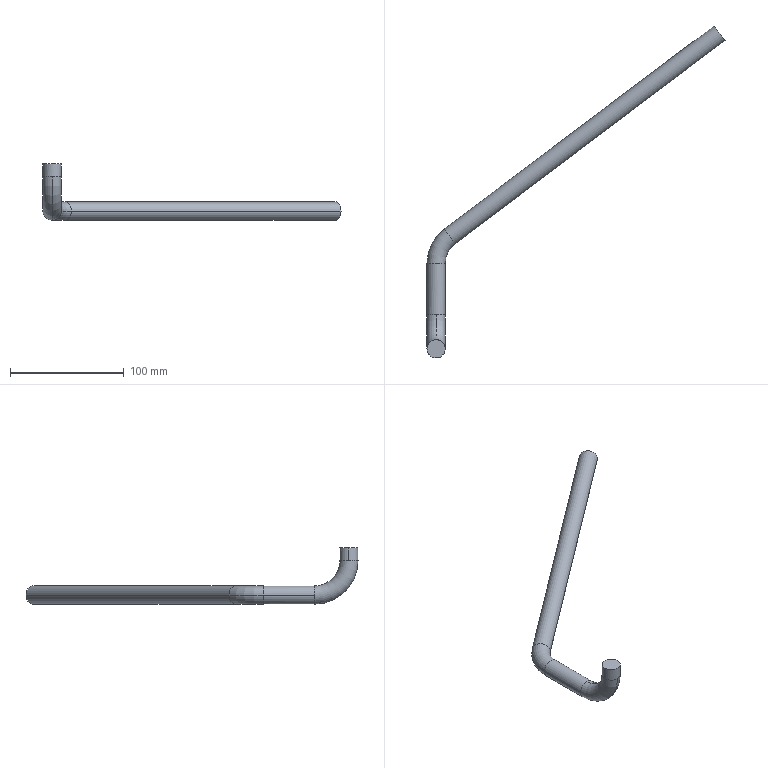Part | STEP file | copper tube 37 | 1 solid | 12 faces | box 261.823 x 291.69 x 49.416 mm | volume 86044 mm3 | cylinder 6 | torus 4 | plane 2 | commonest cylinder face diameters 16 x6
STEP:
#1=CARTESIAN_POINT('',(0.,0.,0.));
#2=DIRECTION('',(0.,0.,1.));
#3=DIRECTION('',(1.,0.,0.));
#4=AXIS2_PLACEMENT_3D('',#1,#2,#3);
#5=CARTESIAN_POINT('',(0.,-8.,-61.416));
#6=VERTEX_POINT('',#5);
#7=CARTESIAN_POINT('',(8.,0.,-61.416));
#8=VERTEX_POINT('',#7);
#9=CARTESIAN_POINT('',(0.,0.,-61.416));
#10=DIRECTION('',(0.,0.,1.));
#11=DIRECTION('',(1.,0.,0.));
#12=AXIS2_PLACEMENT_3D('',#9,#10,#11);
#13=CIRCLE('',#12,8.);
#14=CARTESIAN_POINT('',(0.,30.,-61.416));
#15=DIRECTION('',(1.,0.,0.));
#16=DIRECTION('',(0.,1.,0.));
#17=AXIS2_PLACEMENT_3D('',#14,#15,#16);
#18=TOROIDAL_SURFACE('',#17,30.,8.);
#19=CARTESIAN_POINT('',(3.142,-4.712));
#20=DIRECTION('',(0.,1.));
#21=VECTOR('',#20,1.);
#22=LINE('',#19,#21);
#23=(GEOMETRIC_REPRESENTATION_CONTEXT(2)PARAMETRIC_REPRESENTATION_CONTEXT()REPRESENTATION_CONTEXT('',''));
#24=DEFINITIONAL_REPRESENTATION('',(#22),#23);
#25=PCURVE('',#18,#24);
#26=CARTESIAN_POINT('',(0.,0.,-61.416));
#27=DIRECTION('',(0.,0.,1.));
#28=DIRECTION('',(1.,0.,0.));
#29=AXIS2_PLACEMENT_3D('',#26,#27,#28);
#30=CYLINDRICAL_SURFACE('',#29,8.);
#31=CARTESIAN_POINT('',(0.,0.));
#32=DIRECTION('',(1.,0.));
#33=VECTOR('',#32,1.);
#34=LINE('',#31,#33);
#35=(GEOMETRIC_REPRESENTATION_CONTEXT(2)PARAMETRIC_REPRESENTATION_CONTEXT()REPRESENTATION_CONTEXT('',''));
#36=DEFINITIONAL_REPRESENTATION('',(#34),#35);
#37=PCURVE('',#30,#36);
#38=SURFACE_CURVE('',#13,(#25,#37),.PCURVE_S1.);
#39=EDGE_CURVE('',#6,#8,#38,.T.);
#40=ORIENTED_EDGE('',*,*,#39,.F.);
#41=CARTESIAN_POINT('',(0.,30.,-99.416));
#42=VERTEX_POINT('',#41);
#43=CARTESIAN_POINT('',(0.,30.,-61.416));
#44=DIRECTION('',(1.,0.,0.));
#45=DIRECTION('',(0.,1.,0.));
#46=AXIS2_PLACEMENT_3D('',#43,#44,#45);
#47=CIRCLE('',#46,38.);
#48=CARTESIAN_POINT('',(0.,0.));
#49=DIRECTION('',(1.,0.));
#50=VECTOR('',#49,1.);
#51=LINE('',#48,#50);
#52=(GEOMETRIC_REPRESENTATION_CONTEXT(2)PARAMETRIC_REPRESENTATION_CONTEXT()REPRESENTATION_CONTEXT('',''));
#53=DEFINITIONAL_REPRESENTATION('',(#51),#52);
#54=PCURVE('',#18,#53);
#55=CARTESIAN_POINT('',(0.,30.,-61.416));
#56=DIRECTION('',(1.,0.,0.));
#57=DIRECTION('',(0.,1.,0.));
#58=AXIS2_PLACEMENT_3D('',#55,#56,#57);
#59=TOROIDAL_SURFACE('',#58,30.,8.);
#60=CARTESIAN_POINT('',(0.,6.283));
#61=DIRECTION('',(1.,0.));
#62=VECTOR('',#61,1.);
#63=LINE('',#60,#62);
#64=(GEOMETRIC_REPRESENTATION_CONTEXT(2)PARAMETRIC_REPRESENTATION_CONTEXT()REPRESENTATION_CONTEXT('',''));
#65=DEFINITIONAL_REPRESENTATION('',(#63),#64);
#66=PCURVE('',#59,#65);
#67=SURFACE_CURVE('',#47,(#54,#66),.PCURVE_S1.);
#68=EDGE_CURVE('',#6,#42,#67,.T.);
#69=ORIENTED_EDGE('',*,*,#68,.T.);
#70=CARTESIAN_POINT('',(8.,30.,-91.416));
#71=VERTEX_POINT('',#70);
#72=CARTESIAN_POINT('',(0.,30.,-91.416));
#73=DIRECTION('',(0.,-1.,0.));
#74=DIRECTION('',(1.,0.,0.));
#75=AXIS2_PLACEMENT_3D('',#72,#73,#74);
#76=CIRCLE('',#75,8.);
#77=CARTESIAN_POINT('',(4.712,-4.712));
#78=DIRECTION('',(0.,1.));
#79=VECTOR('',#78,1.);
#80=LINE('',#77,#79);
#81=(GEOMETRIC_REPRESENTATION_CONTEXT(2)PARAMETRIC_REPRESENTATION_CONTEXT()REPRESENTATION_CONTEXT('',''));
#82=DEFINITIONAL_REPRESENTATION('',(#80),#81);
#83=PCURVE('',#18,#82);
#84=CARTESIAN_POINT('',(0.,30.,-91.416));
#85=DIRECTION('',(0.,1.,0.));
#86=DIRECTION('',(-1.,0.,0.));
#87=AXIS2_PLACEMENT_3D('',#84,#85,#86);
#88=CYLINDRICAL_SURFACE('',#87,8.);
#89=CARTESIAN_POINT('',(9.425,0.));
#90=DIRECTION('',(-1.,0.));
#91=VECTOR('',#90,1.);
#92=LINE('',#89,#91);
#93=(GEOMETRIC_REPRESENTATION_CONTEXT(2)PARAMETRIC_REPRESENTATION_CONTEXT()REPRESENTATION_CONTEXT('',''));
#94=DEFINITIONAL_REPRESENTATION('',(#92),#93);
#95=PCURVE('',#88,#94);
#96=SURFACE_CURVE('',#76,(#83,#95),.PCURVE_S1.);
#97=EDGE_CURVE('',#42,#71,#96,.T.);
#98=ORIENTED_EDGE('',*,*,#97,.T.);
#99=CARTESIAN_POINT('',(0.,30.,-83.416));
#100=VERTEX_POINT('',#99);
#101=CARTESIAN_POINT('',(0.,30.,-91.416));
#102=DIRECTION('',(0.,-1.,0.));
#103=DIRECTION('',(1.,0.,0.));
#104=AXIS2_PLACEMENT_3D('',#101,#102,#103);
#105=CIRCLE('',#104,8.);
#106=CARTESIAN_POINT('',(4.712,1.571));
#107=DIRECTION('',(0.,1.));
#108=VECTOR('',#107,1.);
#109=LINE('',#106,#108);
#110=(GEOMETRIC_REPRESENTATION_CONTEXT(2)PARAMETRIC_REPRESENTATION_CONTEXT()REPRESENTATION_CONTEXT('',''));
#111=DEFINITIONAL_REPRESENTATION('',(#109),#110);
#112=PCURVE('',#18,#111);
#113=CARTESIAN_POINT('',(0.,30.,-91.416));
#114=DIRECTION('',(0.,1.,0.));
#115=DIRECTION('',(-1.,0.,0.));
#116=AXIS2_PLACEMENT_3D('',#113,#114,#115);
#117=CYLINDRICAL_SURFACE('',#116,8.);
#118=CARTESIAN_POINT('',(3.142,0.));
#119=DIRECTION('',(-1.,0.));
#120=VECTOR('',#119,1.);
#121=LINE('',#118,#120);
#122=(GEOMETRIC_REPRESENTATION_CONTEXT(2)PARAMETRIC_REPRESENTATION_CONTEXT()REPRESENTATION_CONTEXT('',''));
#123=DEFINITIONAL_REPRESENTATION('',(#121),#122);
#124=PCURVE('',#117,#123);
#125=SURFACE_CURVE('',#105,(#112,#124),.PCURVE_S1.);
#126=EDGE_CURVE('',#71,#100,#125,.T.);
#127=ORIENTED_EDGE('',*,*,#126,.T.);
#128=CARTESIAN_POINT('',(0.,8.,-61.416));
#129=VERTEX_POINT('',#128);
#130=CARTESIAN_POINT('',(0.,30.,-61.416));
#131=DIRECTION('',(1.,0.,0.));
#132=DIRECTION('',(0.,1.,0.));
#133=AXIS2_PLACEMENT_3D('',#130,#131,#132);
#134=CIRCLE('',#133,22.);
#135=CARTESIAN_POINT('',(0.,3.142));
#136=DIRECTION('',(1.,0.));
#137=VECTOR('',#136,1.);
#138=LINE('',#135,#137);
#139=(GEOMETRIC_REPRESENTATION_CONTEXT(2)PARAMETRIC_REPRESENTATION_CONTEXT()REPRESENTATION_CONTEXT('',''));
#140=DEFINITIONAL_REPRESENTATION('',(#138),#139);
#141=PCURVE('',#18,#140);
#142=CARTESIAN_POINT('',(0.,3.142));
#143=DIRECTION('',(1.,0.));
#144=VECTOR('',#143,1.);
#145=LINE('',#142,#144);
#146=(GEOMETRIC_REPRESENTATION_CONTEXT(2)PARAMETRIC_REPRESENTATION_CONTEXT()REPRESENTATION_CONTEXT('',''));
#147=DEFINITIONAL_REPRESENTATION('',(#145),#146);
#148=PCURVE('',#59,#147);
#149=SURFACE_CURVE('',#134,(#141,#148),.PCURVE_S1.);
#150=EDGE_CURVE('',#129,#100,#149,.T.);
#151=ORIENTED_EDGE('',*,*,#150,.F.);
#152=CARTESIAN_POINT('',(0.,0.,-61.416));
#153=DIRECTION('',(0.,0.,1.));
#154=DIRECTION('',(1.,0.,0.));
#155=AXIS2_PLACEMENT_3D('',#152,#153,#154);
#156=CIRCLE('',#155,8.);
#157=CARTESIAN_POINT('',(3.142,1.571));
#158=DIRECTION('',(0.,1.));
#159=VECTOR('',#158,1.);
#160=LINE('',#157,#159);
#161=(GEOMETRIC_REPRESENTATION_CONTEXT(2)PARAMETRIC_REPRESENTATION_CONTEXT()REPRESENTATION_CONTEXT('',''));
#162=DEFINITIONAL_REPRESENTATION('',(#160),#161);
#163=PCURVE('',#18,#162);
#164=CARTESIAN_POINT('',(0.,0.,-61.416));
#165=DIRECTION('',(0.,0.,1.));
#166=DIRECTION('',(1.,0.,0.));
#167=AXIS2_PLACEMENT_3D('',#164,#165,#166);
#168=CYLINDRICAL_SURFACE('',#167,8.);
#169=CARTESIAN_POINT('',(0.,0.));
#170=DIRECTION('',(1.,0.));
#171=VECTOR('',#170,1.);
#172=LINE('',#169,#171);
#173=(GEOMETRIC_REPRESENTATION_CONTEXT(2)PARAMETRIC_REPRESENTATION_CONTEXT()REPRESENTATION_CONTEXT('',''));
#174=DEFINITIONAL_REPRESENTATION('',(#172),#173);
#175=PCURVE('',#168,#174);
#176=SURFACE_CURVE('',#156,(#163,#175),.PCURVE_S1.);
#177=EDGE_CURVE('',#8,#129,#176,.T.);
#178=ORIENTED_EDGE('',*,*,#177,.F.);
#179=EDGE_LOOP('',(#40,#69,#98,#127,#151,#178));
#180=FACE_BOUND('',#179,.T.);
#181=ADVANCED_FACE('',(#180),#18,.T.);
#182=CARTESIAN_POINT('',(-8.,75.,-91.416));
#183=VERTEX_POINT('',#182);
#184=CARTESIAN_POINT('',(8.,75.,-91.416));
#185=VERTEX_POINT('',#184);
#186=CARTESIAN_POINT('',(0.,75.,-91.416));
#187=DIRECTION('',(0.,-1.,0.));
#188=DIRECTION('',(1.,0.,0.));
#189=AXIS2_PLACEMENT_3D('',#186,#187,#188);
#190=CIRCLE('',#189,8.);
#191=CARTESIAN_POINT('',(30.,75.,-91.416));
#192=DIRECTION('',(0.,0.,-1.));
#193=DIRECTION('',(-1.,0.,0.));
#194=AXIS2_PLACEMENT_3D('',#191,#192,#193);
#195=TOROIDAL_SURFACE('',#194,30.,8.);
#196=CARTESIAN_POINT('',(0.,-3.142));
#197=DIRECTION('',(0.,1.));
#198=VECTOR('',#197,1.);
#199=LINE('',#196,#198);
#200=(GEOMETRIC_REPRESENTATION_CONTEXT(2)PARAMETRIC_REPRESENTATION_CONTEXT()REPRESENTATION_CONTEXT('',''));
#201=DEFINITIONAL_REPRESENTATION('',(#199),#200);
#202=PCURVE('',#195,#201);
#203=CARTESIAN_POINT('',(9.425,45.));
#204=DIRECTION('',(-1.,0.));
#205=VECTOR('',#204,1.);
#206=LINE('',#203,#205);
#207=(GEOMETRIC_REPRESENTATION_CONTEXT(2)PARAMETRIC_REPRESENTATION_CONTEXT()REPRESENTATION_CONTEXT('',''));
#208=DEFINITIONAL_REPRESENTATION('',(#206),#207);
#209=PCURVE('',#88,#208);
#210=SURFACE_CURVE('',#190,(#202,#209),.PCURVE_S1.);
#211=EDGE_CURVE('',#183,#185,#210,.T.);
#212=ORIENTED_EDGE('',*,*,#211,.F.);
#213=CARTESIAN_POINT('',(7.156,105.367,-91.416));
#214=VERTEX_POINT('',#213);
#215=CARTESIAN_POINT('',(30.,75.,-91.416));
#216=DIRECTION('',(0.,0.,-1.));
#217=DIRECTION('',(-1.,0.,0.));
#218=AXIS2_PLACEMENT_3D('',#215,#216,#217);
#219=CIRCLE('',#218,38.);
#220=CARTESIAN_POINT('',(0.,0.));
#221=DIRECTION('',(1.,0.));
#222=VECTOR('',#221,1.);
#223=LINE('',#220,#222);
#224=(GEOMETRIC_REPRESENTATION_CONTEXT(2)PARAMETRIC_REPRESENTATION_CONTEXT()REPRESENTATION_CONTEXT('',''));
#225=DEFINITIONAL_REPRESENTATION('',(#223),#224);
#226=PCURVE('',#195,#225);
#227=CARTESIAN_POINT('',(30.,75.,-91.416));
#228=DIRECTION('',(0.,0.,-1.));
#229=DIRECTION('',(-1.,0.,0.));
#230=AXIS2_PLACEMENT_3D('',#227,#228,#229);
#231=TOROIDAL_SURFACE('',#230,30.,8.);
#232=CARTESIAN_POINT('',(0.,6.283));
#233=DIRECTION('',(1.,0.));
#234=VECTOR('',#233,1.);
#235=LINE('',#232,#234);
#236=(GEOMETRIC_REPRESENTATION_CONTEXT(2)PARAMETRIC_REPRESENTATION_CONTEXT()REPRESENTATION_CONTEXT('',''));
#237=DEFINITIONAL_REPRESENTATION('',(#235),#236);
#238=PCURVE('',#231,#237);
#239=SURFACE_CURVE('',#219,(#226,#238),.PCURVE_S1.);
#240=EDGE_CURVE('',#183,#214,#239,.T.);
#241=ORIENTED_EDGE('',*,*,#240,.T.);
#242=CARTESIAN_POINT('',(16.775,92.581,-91.416));
#243=VERTEX_POINT('',#242);
#244=CARTESIAN_POINT('',(11.965,98.974,-91.416));
#245=DIRECTION('',(-0.7991,-0.6012,0.));
#246=DIRECTION('',(0.6012,-0.7991,0.));
#247=AXIS2_PLACEMENT_3D('',#244,#245,#246);
#248=CIRCLE('',#247,8.);
#249=CARTESIAN_POINT('',(0.9258,-3.142));
#250=DIRECTION('',(0.,1.));
#251=VECTOR('',#250,1.);
#252=LINE('',#249,#251);
#253=(GEOMETRIC_REPRESENTATION_CONTEXT(2)PARAMETRIC_REPRESENTATION_CONTEXT()REPRESENTATION_CONTEXT('',''));
#254=DEFINITIONAL_REPRESENTATION('',(#252),#253);
#255=PCURVE('',#195,#254);
#256=CARTESIAN_POINT('',(11.965,98.974,-91.416));
#257=DIRECTION('',(0.7991,0.6012,0.));
#258=DIRECTION('',(-0.6012,0.7991,0.));
#259=AXIS2_PLACEMENT_3D('',#256,#257,#258);
#260=CYLINDRICAL_SURFACE('',#259,8.);
#261=CARTESIAN_POINT('',(9.425,0.));
#262=DIRECTION('',(-1.,0.));
#263=VECTOR('',#262,1.);
#264=LINE('',#261,#263);
#265=(GEOMETRIC_REPRESENTATION_CONTEXT(2)PARAMETRIC_REPRESENTATION_CONTEXT()REPRESENTATION_CONTEXT('',''));
#266=DEFINITIONAL_REPRESENTATION('',(#264),#265);
#267=PCURVE('',#260,#266);
#268=SURFACE_CURVE('',#248,(#255,#267),.PCURVE_S1.);
#269=EDGE_CURVE('',#214,#243,#268,.T.);
#270=ORIENTED_EDGE('',*,*,#269,.T.);
#271=CARTESIAN_POINT('',(30.,75.,-91.416));
#272=DIRECTION('',(0.,0.,-1.));
#273=DIRECTION('',(-1.,0.,0.));
#274=AXIS2_PLACEMENT_3D('',#271,#272,#273);
#275=CIRCLE('',#274,22.);
#276=CARTESIAN_POINT('',(0.,3.142));
#277=DIRECTION('',(1.,0.));
#278=VECTOR('',#277,1.);
#279=LINE('',#276,#278);
#280=(GEOMETRIC_REPRESENTATION_CONTEXT(2)PARAMETRIC_REPRESENTATION_CONTEXT()REPRESENTATION_CONTEXT('',''));
#281=DEFINITIONAL_REPRESENTATION('',(#279),#280);
#282=PCURVE('',#195,#281);
#283=CARTESIAN_POINT('',(0.,3.142));
#284=DIRECTION('',(1.,0.));
#285=VECTOR('',#284,1.);
#286=LINE('',#283,#285);
#287=(GEOMETRIC_REPRESENTATION_CONTEXT(2)PARAMETRIC_REPRESENTATION_CONTEXT()REPRESENTATION_CONTEXT('',''));
#288=DEFINITIONAL_REPRESENTATION('',(#286),#287);
#289=PCURVE('',#231,#288);
#290=SURFACE_CURVE('',#275,(#282,#289),.PCURVE_S1.);
#291=EDGE_CURVE('',#185,#243,#290,.T.);
#292=ORIENTED_EDGE('',*,*,#291,.F.);
#293=EDGE_LOOP('',(#212,#241,#270,#292));
#294=FACE_BOUND('',#293,.T.);
#295=ADVANCED_FACE('',(#294),#195,.T.);
#296=ORIENTED_EDGE('',*,*,#126,.F.);
#297=CARTESIAN_POINT('',(8.,30.,-91.416));
#298=DIRECTION('',(0.,1.,0.));
#299=VECTOR('',#298,1.);
#300=LINE('',#297,#299);
#301=CARTESIAN_POINT('',(3.142,0.));
#302=DIRECTION('',(0.,1.));
#303=VECTOR('',#302,1.);
#304=LINE('',#301,#303);
#305=(GEOMETRIC_REPRESENTATION_CONTEXT(2)PARAMETRIC_REPRESENTATION_CONTEXT()REPRESENTATION_CONTEXT('',''));
#306=DEFINITIONAL_REPRESENTATION('',(#304),#305);
#307=PCURVE('',#117,#306);
#308=CARTESIAN_POINT('',(3.142,0.));
#309=DIRECTION('',(0.,1.));
#310=VECTOR('',#309,1.);
#311=LINE('',#308,#310);
#312=(GEOMETRIC_REPRESENTATION_CONTEXT(2)PARAMETRIC_REPRESENTATION_CONTEXT()REPRESENTATION_CONTEXT('',''));
#313=DEFINITIONAL_REPRESENTATION('',(#311),#312);
#314=PCURVE('',#88,#313);
#315=SURFACE_CURVE('',#300,(#307,#314),.PCURVE_S1.);
#316=EDGE_CURVE('',#71,#185,#315,.T.);
#317=ORIENTED_EDGE('',*,*,#316,.T.);
#318=CARTESIAN_POINT('',(0.,75.,-91.416));
#319=DIRECTION('',(0.,-1.,0.));
#320=DIRECTION('',(1.,0.,0.));
#321=AXIS2_PLACEMENT_3D('',#318,#319,#320);
#322=CIRCLE('',#321,8.);
#323=CARTESIAN_POINT('',(3.142,45.));
#324=DIRECTION('',(-1.,0.));
#325=VECTOR('',#324,1.);
#326=LINE('',#323,#325);
#327=(GEOMETRIC_REPRESENTATION_CONTEXT(2)PARAMETRIC_REPRESENTATION_CONTEXT()REPRESENTATION_CONTEXT('',''));
#328=DEFINITIONAL_REPRESENTATION('',(#326),#327);
#329=PCURVE('',#117,#328);
#330=CARTESIAN_POINT('',(0.,3.142));
#331=DIRECTION('',(0.,1.));
#332=VECTOR('',#331,1.);
#333=LINE('',#330,#332);
#334=(GEOMETRIC_REPRESENTATION_CONTEXT(2)PARAMETRIC_REPRESENTATION_CONTEXT()REPRESENTATION_CONTEXT('',''));
#335=DEFINITIONAL_REPRESENTATION('',(#333),#334);
#336=PCURVE('',#231,#335);
#337=SURFACE_CURVE('',#322,(#329,#336),.PCURVE_S1.);
#338=EDGE_CURVE('',#185,#183,#337,.T.);
#339=ORIENTED_EDGE('',*,*,#338,.T.);
#340=CARTESIAN_POINT('',(-8.,30.,-91.416));
#341=VERTEX_POINT('',#340);
#342=CARTESIAN_POINT('',(-8.,30.,-91.416));
#343=DIRECTION('',(0.,1.,0.));
#344=VECTOR('',#343,1.);
#345=LINE('',#342,#344);
#346=CARTESIAN_POINT('',(0.,0.));
#347=DIRECTION('',(0.,1.));
#348=VECTOR('',#347,1.);
#349=LINE('',#346,#348);
#350=(GEOMETRIC_REPRESENTATION_CONTEXT(2)PARAMETRIC_REPRESENTATION_CONTEXT()REPRESENTATION_CONTEXT('',''));
#351=DEFINITIONAL_REPRESENTATION('',(#349),#350);
#352=PCURVE('',#117,#351);
#353=CARTESIAN_POINT('',(6.283,0.));
#354=DIRECTION('',(0.,1.));
#355=VECTOR('',#354,1.);
#356=LINE('',#353,#355);
#357=(GEOMETRIC_REPRESENTATION_CONTEXT(2)PARAMETRIC_REPRESENTATION_CONTEXT()REPRESENTATION_CONTEXT('',''));
#358=DEFINITIONAL_REPRESENTATION('',(#356),#357);
#359=PCURVE('',#88,#358);
#360=SURFACE_CURVE('',#345,(#352,#359),.PCURVE_S1.);
#361=EDGE_CURVE('',#341,#183,#360,.T.);
#362=ORIENTED_EDGE('',*,*,#361,.F.);
#363=CARTESIAN_POINT('',(0.,30.,-91.416));
#364=DIRECTION('',(0.,-1.,0.));
#365=DIRECTION('',(1.,0.,0.));
#366=AXIS2_PLACEMENT_3D('',#363,#364,#365);
#367=CIRCLE('',#366,8.);
#368=CARTESIAN_POINT('',(3.142,0.));
#369=DIRECTION('',(-1.,0.));
#370=VECTOR('',#369,1.);
#371=LINE('',#368,#370);
#372=(GEOMETRIC_REPRESENTATION_CONTEXT(2)PARAMETRIC_REPRESENTATION_CONTEXT()REPRESENTATION_CONTEXT('',''));
#373=DEFINITIONAL_REPRESENTATION('',(#371),#372);
#374=PCURVE('',#117,#373);
#375=CARTESIAN_POINT('',(4.712,1.571));
#376=DIRECTION('',(0.,1.));
#377=VECTOR('',#376,1.);
#378=LINE('',#375,#377);
#379=(GEOMETRIC_REPRESENTATION_CONTEXT(2)PARAMETRIC_REPRESENTATION_CONTEXT()REPRESENTATION_CONTEXT('',''));
#380=DEFINITIONAL_REPRESENTATION('',(#378),#379);
#381=PCURVE('',#59,#380);
#382=SURFACE_CURVE('',#367,(#374,#381),.PCURVE_S1.);
#383=EDGE_CURVE('',#100,#341,#382,.T.);
#384=ORIENTED_EDGE('',*,*,#383,.F.);
#385=EDGE_LOOP('',(#296,#317,#339,#362,#384));
#386=FACE_BOUND('',#385,.T.);
#387=ADVANCED_FACE('',(#386),#117,.T.);
#388=CARTESIAN_POINT('',(11.965,98.974,-91.416));
#389=DIRECTION('',(-0.7991,-0.6012,0.));
#390=DIRECTION('',(0.6012,-0.7991,0.));
#391=AXIS2_PLACEMENT_3D('',#388,#389,#390);
#392=CIRCLE('',#391,8.);
#393=CARTESIAN_POINT('',(11.965,98.974,-91.416));
#394=DIRECTION('',(0.7991,0.6012,0.));
#395=DIRECTION('',(-0.6012,0.7991,0.));
#396=AXIS2_PLACEMENT_3D('',#393,#394,#395);
#397=CYLINDRICAL_SURFACE('',#396,8.);
#398=CARTESIAN_POINT('',(3.142,0.));
#399=DIRECTION('',(-1.,0.));
#400=VECTOR('',#399,1.);
#401=LINE('',#398,#400);
#402=(GEOMETRIC_REPRESENTATION_CONTEXT(2)PARAMETRIC_REPRESENTATION_CONTEXT()REPRESENTATION_CONTEXT('',''));
#403=DEFINITIONAL_REPRESENTATION('',(#401),#402);
#404=PCURVE('',#397,#403);
#405=CARTESIAN_POINT('',(0.9258,3.142));
#406=DIRECTION('',(0.,1.));
#407=VECTOR('',#406,1.);
#408=LINE('',#405,#407);
#409=(GEOMETRIC_REPRESENTATION_CONTEXT(2)PARAMETRIC_REPRESENTATION_CONTEXT()REPRESENTATION_CONTEXT('',''));
#410=DEFINITIONAL_REPRESENTATION('',(#408),#409);
#411=PCURVE('',#231,#410);
#412=SURFACE_CURVE('',#392,(#404,#411),.PCURVE_S1.);
#413=EDGE_CURVE('',#243,#214,#412,.T.);
#414=ORIENTED_EDGE('',*,*,#413,.F.);
#415=CARTESIAN_POINT('',(253.823,270.904,-91.416));
#416=VERTEX_POINT('',#415);
#417=CARTESIAN_POINT('',(16.775,92.581,-91.416));
#418=DIRECTION('',(0.7991,0.6012,0.));
#419=VECTOR('',#418,1.);
#420=LINE('',#417,#419);
#421=CARTESIAN_POINT('',(3.142,0.));
#422=DIRECTION('',(0.,1.));
#423=VECTOR('',#422,1.);
#424=LINE('',#421,#423);
#425=(GEOMETRIC_REPRESENTATION_CONTEXT(2)PARAMETRIC_REPRESENTATION_CONTEXT()REPRESENTATION_CONTEXT('',''));
#426=DEFINITIONAL_REPRESENTATION('',(#424),#425);
#427=PCURVE('',#397,#426);
#428=CARTESIAN_POINT('',(3.142,0.));
#429=DIRECTION('',(0.,1.));
#430=VECTOR('',#429,1.);
#431=LINE('',#428,#430);
#432=(GEOMETRIC_REPRESENTATION_CONTEXT(2)PARAMETRIC_REPRESENTATION_CONTEXT()REPRESENTATION_CONTEXT('',''));
#433=DEFINITIONAL_REPRESENTATION('',(#431),#432);
#434=PCURVE('',#260,#433);
#435=SURFACE_CURVE('',#420,(#427,#434),.PCURVE_S1.);
#436=EDGE_CURVE('',#243,#416,#435,.T.);
#437=ORIENTED_EDGE('',*,*,#436,.T.);
#438=CARTESIAN_POINT('',(244.205,283.69,-91.416));
#439=VERTEX_POINT('',#438);
#440=CARTESIAN_POINT('',(249.014,277.297,-91.416));
#441=DIRECTION('',(-0.7991,-0.6012,0.));
#442=DIRECTION('',(0.6012,-0.7991,0.));
#443=AXIS2_PLACEMENT_3D('',#440,#441,#442);
#444=CIRCLE('',#443,8.);
#445=CARTESIAN_POINT('',(3.142,296.633));
#446=DIRECTION('',(-1.,0.));
#447=VECTOR('',#446,1.);
#448=LINE('',#445,#447);
#449=(GEOMETRIC_REPRESENTATION_CONTEXT(2)PARAMETRIC_REPRESENTATION_CONTEXT()REPRESENTATION_CONTEXT('',''));
#450=DEFINITIONAL_REPRESENTATION('',(#448),#449);
#451=PCURVE('',#397,#450);
#452=CARTESIAN_POINT('',(249.014,277.297,-91.416));
#453=DIRECTION('',(-0.7991,-0.6012,0.));
#454=DIRECTION('',(0.6012,-0.7991,0.));
#455=AXIS2_PLACEMENT_3D('',#452,#453,#454);
#456=PLANE('',#455);
#457=CARTESIAN_POINT('',(0.,0.));
#458=DIRECTION('',(1.,0.));
#459=AXIS2_PLACEMENT_2D('',#457,#458);
#460=CIRCLE('',#459,8.);
#461=(GEOMETRIC_REPRESENTATION_CONTEXT(2)PARAMETRIC_REPRESENTATION_CONTEXT()REPRESENTATION_CONTEXT('',''));
#462=DEFINITIONAL_REPRESENTATION('',(#460),#461);
#463=PCURVE('',#456,#462);
#464=SURFACE_CURVE('',#444,(#451,#463),.PCURVE_S1.);
#465=EDGE_CURVE('',#416,#439,#464,.T.);
#466=ORIENTED_EDGE('',*,*,#465,.T.);
#467=CARTESIAN_POINT('',(7.156,105.367,-91.416));
#468=DIRECTION('',(0.7991,0.6012,0.));
#469=VECTOR('',#468,1.);
#470=LINE('',#467,#469);
#471=CARTESIAN_POINT('',(0.,0.));
#472=DIRECTION('',(0.,1.));
#473=VECTOR('',#472,1.);
#474=LINE('',#471,#473);
#475=(GEOMETRIC_REPRESENTATION_CONTEXT(2)PARAMETRIC_REPRESENTATION_CONTEXT()REPRESENTATION_CONTEXT('',''));
#476=DEFINITIONAL_REPRESENTATION('',(#474),#475);
#477=PCURVE('',#397,#476);
#478=CARTESIAN_POINT('',(6.283,0.));
#479=DIRECTION('',(0.,1.));
#480=VECTOR('',#479,1.);
#481=LINE('',#478,#480);
#482=(GEOMETRIC_REPRESENTATION_CONTEXT(2)PARAMETRIC_REPRESENTATION_CONTEXT()REPRESENTATION_CONTEXT('',''));
#483=DEFINITIONAL_REPRESENTATION('',(#481),#482);
#484=PCURVE('',#260,#483);
#485=SURFACE_CURVE('',#470,(#477,#484),.PCURVE_S1.);
#486=EDGE_CURVE('',#214,#439,#485,.T.);
#487=ORIENTED_EDGE('',*,*,#486,.F.);
#488=EDGE_LOOP('',(#414,#437,#466,#487));
#489=FACE_BOUND('',#488,.T.);
#490=ADVANCED_FACE('',(#489),#397,.T.);
#491=ORIENTED_EDGE('',*,*,#177,.T.);
#492=CARTESIAN_POINT('',(-8.,0.,-61.416));
#493=VERTEX_POINT('',#492);
#494=CARTESIAN_POINT('',(0.,0.,-61.416));
#495=DIRECTION('',(0.,0.,1.));
#496=DIRECTION('',(1.,0.,0.));
#497=AXIS2_PLACEMENT_3D('',#494,#495,#496);
#498=CIRCLE('',#497,8.);
#499=CARTESIAN_POINT('',(0.,0.));
#500=DIRECTION('',(1.,0.));
#501=VECTOR('',#500,1.);
#502=LINE('',#499,#501);
#503=(GEOMETRIC_REPRESENTATION_CONTEXT(2)PARAMETRIC_REPRESENTATION_CONTEXT()REPRESENTATION_CONTEXT('',''));
#504=DEFINITIONAL_REPRESENTATION('',(#502),#503);
#505=PCURVE('',#168,#504);
#506=CARTESIAN_POINT('',(3.142,1.571));
#507=DIRECTION('',(0.,1.));
#508=VECTOR('',#507,1.);
#509=LINE('',#506,#508);
#510=(GEOMETRIC_REPRESENTATION_CONTEXT(2)PARAMETRIC_REPRESENTATION_CONTEXT()REPRESENTATION_CONTEXT('',''));
#511=DEFINITIONAL_REPRESENTATION('',(#509),#510);
#512=PCURVE('',#59,#511);
#513=SURFACE_CURVE('',#498,(#505,#512),.PCURVE_S1.);
#514=EDGE_CURVE('',#129,#493,#513,.T.);
#515=ORIENTED_EDGE('',*,*,#514,.T.);
#516=CARTESIAN_POINT('',(-8.,0.,-50.));
#517=VERTEX_POINT('',#516);
#518=CARTESIAN_POINT('',(-8.,0.,-61.416));
#519=DIRECTION('',(0.,0.,1.));
#520=VECTOR('',#519,1.);
#521=LINE('',#518,#520);
#522=CARTESIAN_POINT('',(3.142,0.));
#523=DIRECTION('',(0.,1.));
#524=VECTOR('',#523,1.);
#525=LINE('',#522,#524);
#526=(GEOMETRIC_REPRESENTATION_CONTEXT(2)PARAMETRIC_REPRESENTATION_CONTEXT()REPRESENTATION_CONTEXT('',''));
#527=DEFINITIONAL_REPRESENTATION('',(#525),#526);
#528=PCURVE('',#168,#527);
#529=CARTESIAN_POINT('',(3.142,0.));
#530=DIRECTION('',(0.,1.));
#531=VECTOR('',#530,1.);
#532=LINE('',#529,#531);
#533=(GEOMETRIC_REPRESENTATION_CONTEXT(2)PARAMETRIC_REPRESENTATION_CONTEXT()REPRESENTATION_CONTEXT('',''));
#534=DEFINITIONAL_REPRESENTATION('',(#532),#533);
#535=PCURVE('',#30,#534);
#536=SURFACE_CURVE('',#521,(#528,#535),.PCURVE_S1.);
#537=EDGE_CURVE('',#493,#517,#536,.T.);
#538=ORIENTED_EDGE('',*,*,#537,.T.);
#539=CARTESIAN_POINT('',(8.,0.,-50.));
#540=VERTEX_POINT('',#539);
#541=CARTESIAN_POINT('',(0.,0.,-50.));
#542=DIRECTION('',(0.,0.,-1.));
#543=DIRECTION('',(1.,0.,0.));
#544=AXIS2_PLACEMENT_3D('',#541,#542,#543);
#545=CIRCLE('',#544,8.);
#546=CARTESIAN_POINT('',(6.283,11.416));
#547=DIRECTION('',(-1.,0.));
#548=VECTOR('',#547,1.);
#549=LINE('',#546,#548);
#550=(GEOMETRIC_REPRESENTATION_CONTEXT(2)PARAMETRIC_REPRESENTATION_CONTEXT()REPRESENTATION_CONTEXT('',''));
#551=DEFINITIONAL_REPRESENTATION('',(#549),#550);
#552=PCURVE('',#168,#551);
#553=CARTESIAN_POINT('',(0.,0.,-50.));
#554=DIRECTION('',(0.,0.,1.));
#555=DIRECTION('',(1.,0.,0.));
#556=AXIS2_PLACEMENT_3D('',#553,#554,#555);
#557=PLANE('',#556);
#558=CARTESIAN_POINT('',(8.,0.));
#559=CARTESIAN_POINT('',(8.,-13.856));
#560=CARTESIAN_POINT('',(-4.,-6.928));
#561=CARTESIAN_POINT('',(-16.,0.));
#562=CARTESIAN_POINT('',(-4.,6.928));
#563=CARTESIAN_POINT('',(8.,13.856));
#564=CARTESIAN_POINT('',(8.,0.));
#565=(BOUNDED_CURVE()B_SPLINE_CURVE(2,(#558,#559,#560,#561,#562,#563,#564),.UNSPECIFIED.,.T.,.F.)B_SPLINE_CURVE_WITH_KNOTS((1,2,2,2,2,1),(-2.094,0.,2.094,4.189,6.283,8.378),.UNSPECIFIED.)CURVE()GEOMETRIC_REPRESENTATION_ITEM()RATIONAL_B_SPLINE_CURVE((1.,0.5,1.,0.5,1.,0.5,1.))REPRESENTATION_ITEM(''));
#566=(GEOMETRIC_REPRESENTATION_CONTEXT(2)PARAMETRIC_REPRESENTATION_CONTEXT()REPRESENTATION_CONTEXT('',''));
#567=DEFINITIONAL_REPRESENTATION('',(#565),#566);
#568=PCURVE('',#557,#567);
#569=SURFACE_CURVE('',#545,(#552,#568),.PCURVE_S1.);
#570=EDGE_CURVE('',#517,#540,#569,.T.);
#571=ORIENTED_EDGE('',*,*,#570,.T.);
#572=CARTESIAN_POINT('',(8.,0.,-61.416));
#573=DIRECTION('',(0.,0.,1.));
#574=VECTOR('',#573,1.);
#575=LINE('',#572,#574);
#576=CARTESIAN_POINT('',(0.,0.));
#577=DIRECTION('',(0.,1.));
#578=VECTOR('',#577,1.);
#579=LINE('',#576,#578);
#580=(GEOMETRIC_REPRESENTATION_CONTEXT(2)PARAMETRIC_REPRESENTATION_CONTEXT()REPRESENTATION_CONTEXT('',''));
#581=DEFINITIONAL_REPRESENTATION('',(#579),#580);
#582=PCURVE('',#168,#581);
#583=CARTESIAN_POINT('',(6.283,0.));
#584=DIRECTION('',(0.,1.));
#585=VECTOR('',#584,1.);
#586=LINE('',#583,#585);
#587=(GEOMETRIC_REPRESENTATION_CONTEXT(2)PARAMETRIC_REPRESENTATION_CONTEXT()REPRESENTATION_CONTEXT('',''));
#588=DEFINITIONAL_REPRESENTATION('',(#586),#587);
#589=PCURVE('',#30,#588);
#590=SURFACE_CURVE('',#575,(#582,#589),.PCURVE_S1.);
#591=EDGE_CURVE('',#8,#540,#590,.T.);
#592=ORIENTED_EDGE('',*,*,#591,.F.);
#593=EDGE_LOOP('',(#491,#515,#538,#571,#592));
#594=FACE_BOUND('',#593,.T.);
#595=ADVANCED_FACE('',(#594),#168,.T.);
#596=ORIENTED_EDGE('',*,*,#537,.F.);
#597=CARTESIAN_POINT('',(0.,0.,-61.416));
#598=DIRECTION('',(0.,0.,1.));
#599=DIRECTION('',(1.,0.,0.));
#600=AXIS2_PLACEMENT_3D('',#597,#598,#599);
#601=CIRCLE('',#600,8.);
#602=CARTESIAN_POINT('',(0.,0.));
#603=DIRECTION('',(1.,0.));
#604=VECTOR('',#603,1.);
#605=LINE('',#602,#604);
#606=(GEOMETRIC_REPRESENTATION_CONTEXT(2)PARAMETRIC_REPRESENTATION_CONTEXT()REPRESENTATION_CONTEXT('',''));
#607=DEFINITIONAL_REPRESENTATION('',(#605),#606);
#608=PCURVE('',#30,#607);
#609=CARTESIAN_POINT('',(3.142,1.571));
#610=DIRECTION('',(0.,1.));
#611=VECTOR('',#610,1.);
#612=LINE('',#609,#611);
#613=(GEOMETRIC_REPRESENTATION_CONTEXT(2)PARAMETRIC_REPRESENTATION_CONTEXT()REPRESENTATION_CONTEXT('',''));
#614=DEFINITIONAL_REPRESENTATION('',(#612),#613);
#615=PCURVE('',#59,#614);
#616=SURFACE_CURVE('',#601,(#608,#615),.PCURVE_S1.);
#617=EDGE_CURVE('',#493,#6,#616,.T.);
#618=ORIENTED_EDGE('',*,*,#617,.T.);
#619=ORIENTED_EDGE('',*,*,#39,.T.);
#620=ORIENTED_EDGE('',*,*,#591,.T.);
#621=CARTESIAN_POINT('',(0.,0.,-50.));
#622=DIRECTION('',(0.,0.,-1.));
#623=DIRECTION('',(1.,0.,0.));
#624=AXIS2_PLACEMENT_3D('',#621,#622,#623);
#625=CIRCLE('',#624,8.);
#626=CARTESIAN_POINT('',(6.283,11.416));
#627=DIRECTION('',(-1.,0.));
#628=VECTOR('',#627,1.);
#629=LINE('',#626,#628);
#630=(GEOMETRIC_REPRESENTATION_CONTEXT(2)PARAMETRIC_REPRESENTATION_CONTEXT()REPRESENTATION_CONTEXT('',''));
#631=DEFINITIONAL_REPRESENTATION('',(#629),#630);
#632=PCURVE('',#30,#631);
#633=CARTESIAN_POINT('',(8.,0.));
#634=CARTESIAN_POINT('',(8.,-13.856));
#635=CARTESIAN_POINT('',(-4.,-6.928));
#636=CARTESIAN_POINT('',(-16.,0.));
#637=CARTESIAN_POINT('',(-4.,6.928));
#638=CARTESIAN_POINT('',(8.,13.856));
#639=CARTESIAN_POINT('',(8.,0.));
#640=(BOUNDED_CURVE()B_SPLINE_CURVE(2,(#633,#634,#635,#636,#637,#638,#639),.UNSPECIFIED.,.T.,.F.)B_SPLINE_CURVE_WITH_KNOTS((1,2,2,2,2,1),(-2.094,0.,2.094,4.189,6.283,8.378),.UNSPECIFIED.)CURVE()GEOMETRIC_REPRESENTATION_ITEM()RATIONAL_B_SPLINE_CURVE((1.,0.5,1.,0.5,1.,0.5,1.))REPRESENTATION_ITEM(''));
#641=(GEOMETRIC_REPRESENTATION_CONTEXT(2)PARAMETRIC_REPRESENTATION_CONTEXT()REPRESENTATION_CONTEXT('',''));
#642=DEFINITIONAL_REPRESENTATION('',(#640),#641);
#643=PCURVE('',#557,#642);
#644=SURFACE_CURVE('',#625,(#632,#643),.PCURVE_S1.);
#645=EDGE_CURVE('',#540,#517,#644,.T.);
#646=ORIENTED_EDGE('',*,*,#645,.T.);
#647=EDGE_LOOP('',(#596,#618,#619,#620,#646));
#648=FACE_BOUND('',#647,.T.);
#649=ADVANCED_FACE('',(#648),#30,.T.);
#650=ORIENTED_EDGE('',*,*,#436,.F.);
#651=ORIENTED_EDGE('',*,*,#269,.F.);
#652=ORIENTED_EDGE('',*,*,#486,.T.);
#653=CARTESIAN_POINT('',(249.014,277.297,-91.416));
#654=DIRECTION('',(-0.7991,-0.6012,0.));
#655=DIRECTION('',(0.6012,-0.7991,0.));
#656=AXIS2_PLACEMENT_3D('',#653,#654,#655);
#657=CIRCLE('',#656,8.);
#658=CARTESIAN_POINT('',(9.425,296.633));
#659=DIRECTION('',(-1.,0.));
#660=VECTOR('',#659,1.);
#661=LINE('',#658,#660);
#662=(GEOMETRIC_REPRESENTATION_CONTEXT(2)PARAMETRIC_REPRESENTATION_CONTEXT()REPRESENTATION_CONTEXT('',''));
#663=DEFINITIONAL_REPRESENTATION('',(#661),#662);
#664=PCURVE('',#260,#663);
#665=CARTESIAN_POINT('',(0.,0.));
#666=DIRECTION('',(1.,0.));
#667=AXIS2_PLACEMENT_2D('',#665,#666);
#668=CIRCLE('',#667,8.);
#669=(GEOMETRIC_REPRESENTATION_CONTEXT(2)PARAMETRIC_REPRESENTATION_CONTEXT()REPRESENTATION_CONTEXT('',''));
#670=DEFINITIONAL_REPRESENTATION('',(#668),#669);
#671=PCURVE('',#456,#670);
#672=SURFACE_CURVE('',#657,(#664,#671),.PCURVE_S1.);
#673=EDGE_CURVE('',#439,#416,#672,.T.);
#674=ORIENTED_EDGE('',*,*,#673,.T.);
#675=EDGE_LOOP('',(#650,#651,#652,#674));
#676=FACE_BOUND('',#675,.T.);
#677=ADVANCED_FACE('',(#676),#260,.T.);
#678=ORIENTED_EDGE('',*,*,#240,.F.);
#679=ORIENTED_EDGE('',*,*,#338,.F.);
#680=ORIENTED_EDGE('',*,*,#291,.T.);
#681=ORIENTED_EDGE('',*,*,#413,.T.);
#682=EDGE_LOOP('',(#678,#679,#680,#681));
#683=FACE_BOUND('',#682,.T.);
#684=ADVANCED_FACE('',(#683),#231,.T.);
#685=ORIENTED_EDGE('',*,*,#316,.F.);
#686=ORIENTED_EDGE('',*,*,#97,.F.);
#687=CARTESIAN_POINT('',(0.,30.,-91.416));
#688=DIRECTION('',(0.,-1.,0.));
#689=DIRECTION('',(1.,0.,0.));
#690=AXIS2_PLACEMENT_3D('',#687,#688,#689);
#691=CIRCLE('',#690,8.);
#692=CARTESIAN_POINT('',(9.425,0.));
#693=DIRECTION('',(-1.,0.));
#694=VECTOR('',#693,1.);
#695=LINE('',#692,#694);
#696=(GEOMETRIC_REPRESENTATION_CONTEXT(2)PARAMETRIC_REPRESENTATION_CONTEXT()REPRESENTATION_CONTEXT('',''));
#697=DEFINITIONAL_REPRESENTATION('',(#695),#696);
#698=PCURVE('',#88,#697);
#699=CARTESIAN_POINT('',(4.712,1.571));
#700=DIRECTION('',(0.,1.));
#701=VECTOR('',#700,1.);
#702=LINE('',#699,#701);
#703=(GEOMETRIC_REPRESENTATION_CONTEXT(2)PARAMETRIC_REPRESENTATION_CONTEXT()REPRESENTATION_CONTEXT('',''));
#704=DEFINITIONAL_REPRESENTATION('',(#702),#703);
#705=PCURVE('',#59,#704);
#706=SURFACE_CURVE('',#691,(#698,#705),.PCURVE_S1.);
#707=EDGE_CURVE('',#341,#42,#706,.T.);
#708=ORIENTED_EDGE('',*,*,#707,.F.);
#709=ORIENTED_EDGE('',*,*,#361,.T.);
#710=ORIENTED_EDGE('',*,*,#211,.T.);
#711=EDGE_LOOP('',(#685,#686,#708,#709,#710));
#712=FACE_BOUND('',#711,.T.);
#713=ADVANCED_FACE('',(#712),#88,.T.);
#714=ORIENTED_EDGE('',*,*,#68,.F.);
#715=ORIENTED_EDGE('',*,*,#617,.F.);
#716=ORIENTED_EDGE('',*,*,#514,.F.);
#717=ORIENTED_EDGE('',*,*,#150,.T.);
#718=ORIENTED_EDGE('',*,*,#383,.T.);
#719=ORIENTED_EDGE('',*,*,#707,.T.);
#720=EDGE_LOOP('',(#714,#715,#716,#717,#718,#719));
#721=FACE_BOUND('',#720,.T.);
#722=ADVANCED_FACE('',(#721),#59,.T.);
#723=ORIENTED_EDGE('',*,*,#673,.F.);
#724=ORIENTED_EDGE('',*,*,#465,.F.);
#725=EDGE_LOOP('',(#723,#724));
#726=FACE_BOUND('',#725,.T.);
#727=ADVANCED_FACE('',(#726),#456,.F.);
#728=ORIENTED_EDGE('',*,*,#645,.F.);
#729=ORIENTED_EDGE('',*,*,#570,.F.);
#730=EDGE_LOOP('',(#728,#729));
#731=FACE_BOUND('',#730,.T.);
#732=ADVANCED_FACE('',(#731),#557,.T.);
#733=CLOSED_SHELL('',(#181,#295,#387,#490,#595,#649,#677,#684,#713,#722,#727,#732));
#734=MANIFOLD_SOLID_BREP('',#733);
#735=(LENGTH_UNIT()NAMED_UNIT(*)SI_UNIT(.MILLI.,.METRE.));
#736=UNCERTAINTY_MEASURE_WITH_UNIT(LENGTH_MEASURE(0.0000001),#735,'','');
#737=(NAMED_UNIT(*)PLANE_ANGLE_UNIT()SI_UNIT($,.RADIAN.));
#738=(NAMED_UNIT(*)SI_UNIT($,.STERADIAN.)SOLID_ANGLE_UNIT());
#739=(GEOMETRIC_REPRESENTATION_CONTEXT(3)GLOBAL_UNCERTAINTY_ASSIGNED_CONTEXT((#736))GLOBAL_UNIT_ASSIGNED_CONTEXT((#735,#737,#738))REPRESENTATION_CONTEXT('',''));
#740=ADVANCED_BREP_SHAPE_REPRESENTATION('',(#4,#734),#739);